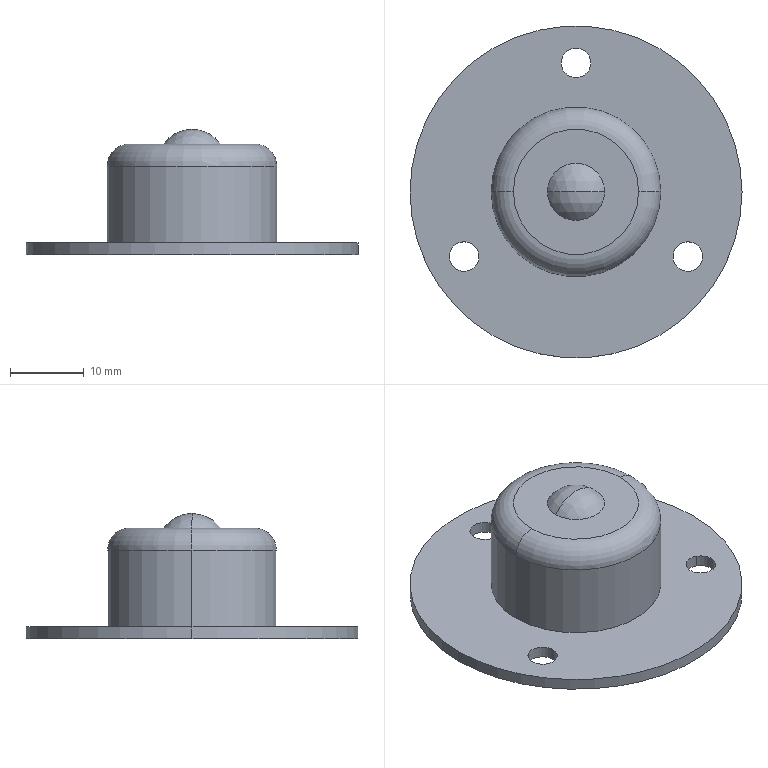Part | STEP file | Caster wheel | 1 solid | 17 faces | box 45 x 45 x 17 mm | volume 7972 mm3 | cylinder 10 | plane 3 | torus 2 | sphere 2 | commonest cylinder face diameters 4 x6 23 x2 45 x2
STEP:
#1=CARTESIAN_POINT('',(0.,0.,0.));
#2=DIRECTION('',(0.,0.,1.));
#3=DIRECTION('',(1.,0.,0.));
#4=AXIS2_PLACEMENT_3D('',#1,#2,#3);
#5=CARTESIAN_POINT('',(-16.155,-7.018,0.));
#6=VERTEX_POINT('',#5);
#7=CARTESIAN_POINT('',(-16.155,-7.018,1.6));
#8=VERTEX_POINT('',#7);
#9=CARTESIAN_POINT('',(-16.155,-7.018,1.6));
#10=DIRECTION('',(0.,0.,1.));
#11=VECTOR('',#10,1.);
#12=LINE('',#9,#11);
#13=CARTESIAN_POINT('',(-15.155,-8.75,1.6));
#14=DIRECTION('',(0.,0.,1.));
#15=DIRECTION('',(-0.5,0.866,0.));
#16=AXIS2_PLACEMENT_3D('',#13,#14,#15);
#17=CYLINDRICAL_SURFACE('',#16,2.);
#18=CARTESIAN_POINT('',(6.283,0.));
#19=DIRECTION('',(0.,1.));
#20=VECTOR('',#19,1.);
#21=LINE('',#18,#20);
#22=(GEOMETRIC_REPRESENTATION_CONTEXT(2)PARAMETRIC_REPRESENTATION_CONTEXT()REPRESENTATION_CONTEXT('',''));
#23=DEFINITIONAL_REPRESENTATION('',(#21),#22);
#24=PCURVE('',#17,#23);
#25=CARTESIAN_POINT('',(-15.155,-8.75,1.6));
#26=DIRECTION('',(0.,0.,1.));
#27=DIRECTION('',(-0.5,0.866,0.));
#28=AXIS2_PLACEMENT_3D('',#25,#26,#27);
#29=CYLINDRICAL_SURFACE('',#28,2.);
#30=CARTESIAN_POINT('',(0.,0.));
#31=DIRECTION('',(0.,1.));
#32=VECTOR('',#31,1.);
#33=LINE('',#30,#32);
#34=(GEOMETRIC_REPRESENTATION_CONTEXT(2)PARAMETRIC_REPRESENTATION_CONTEXT()REPRESENTATION_CONTEXT('',''));
#35=DEFINITIONAL_REPRESENTATION('',(#33),#34);
#36=PCURVE('',#29,#35);
#37=SURFACE_CURVE('',#12,(#24,#36),.PCURVE_S1.);
#38=EDGE_CURVE('',#6,#8,#37,.T.);
#39=ORIENTED_EDGE('',*,*,#38,.T.);
#40=CARTESIAN_POINT('',(-14.155,-10.482,1.6));
#41=VERTEX_POINT('',#40);
#42=CARTESIAN_POINT('',(-15.155,-8.75,1.6));
#43=DIRECTION('',(0.,0.,1.));
#44=DIRECTION('',(-0.5,0.866,0.));
#45=AXIS2_PLACEMENT_3D('',#42,#43,#44);
#46=CIRCLE('',#45,2.);
#47=CARTESIAN_POINT('',(0.,0.));
#48=DIRECTION('',(1.,0.));
#49=VECTOR('',#48,1.);
#50=LINE('',#47,#49);
#51=(GEOMETRIC_REPRESENTATION_CONTEXT(2)PARAMETRIC_REPRESENTATION_CONTEXT()REPRESENTATION_CONTEXT('',''));
#52=DEFINITIONAL_REPRESENTATION('',(#50),#51);
#53=PCURVE('',#17,#52);
#54=CARTESIAN_POINT('',(0.,0.,1.6));
#55=DIRECTION('',(0.,0.,1.));
#56=DIRECTION('',(1.,0.,0.));
#57=AXIS2_PLACEMENT_3D('',#54,#55,#56);
#58=PLANE('',#57);
#59=CARTESIAN_POINT('',(-15.155,-8.75));
#60=DIRECTION('',(-0.5,0.866));
#61=AXIS2_PLACEMENT_2D('',#59,#60);
#62=CIRCLE('',#61,2.);
#63=(GEOMETRIC_REPRESENTATION_CONTEXT(2)PARAMETRIC_REPRESENTATION_CONTEXT()REPRESENTATION_CONTEXT('',''));
#64=DEFINITIONAL_REPRESENTATION('',(#62),#63);
#65=PCURVE('',#58,#64);
#66=SURFACE_CURVE('',#46,(#53,#65),.PCURVE_S1.);
#67=EDGE_CURVE('',#41,#8,#66,.T.);
#68=ORIENTED_EDGE('',*,*,#67,.F.);
#69=CARTESIAN_POINT('',(-14.155,-10.482,0.));
#70=VERTEX_POINT('',#69);
#71=CARTESIAN_POINT('',(-14.155,-10.482,1.6));
#72=DIRECTION('',(0.,0.,1.));
#73=VECTOR('',#72,1.);
#74=LINE('',#71,#73);
#75=CARTESIAN_POINT('',(3.142,0.));
#76=DIRECTION('',(0.,1.));
#77=VECTOR('',#76,1.);
#78=LINE('',#75,#77);
#79=(GEOMETRIC_REPRESENTATION_CONTEXT(2)PARAMETRIC_REPRESENTATION_CONTEXT()REPRESENTATION_CONTEXT('',''));
#80=DEFINITIONAL_REPRESENTATION('',(#78),#79);
#81=PCURVE('',#17,#80);
#82=CARTESIAN_POINT('',(3.142,0.));
#83=DIRECTION('',(0.,1.));
#84=VECTOR('',#83,1.);
#85=LINE('',#82,#84);
#86=(GEOMETRIC_REPRESENTATION_CONTEXT(2)PARAMETRIC_REPRESENTATION_CONTEXT()REPRESENTATION_CONTEXT('',''));
#87=DEFINITIONAL_REPRESENTATION('',(#85),#86);
#88=PCURVE('',#29,#87);
#89=SURFACE_CURVE('',#74,(#81,#88),.PCURVE_S1.);
#90=EDGE_CURVE('',#70,#41,#89,.T.);
#91=ORIENTED_EDGE('',*,*,#90,.F.);
#92=CARTESIAN_POINT('',(-15.155,-8.75,0.));
#93=DIRECTION('',(0.,0.,1.));
#94=DIRECTION('',(-0.5,0.866,0.));
#95=AXIS2_PLACEMENT_3D('',#92,#93,#94);
#96=CIRCLE('',#95,2.);
#97=CARTESIAN_POINT('',(0.,-1.6));
#98=DIRECTION('',(1.,0.));
#99=VECTOR('',#98,1.);
#100=LINE('',#97,#99);
#101=(GEOMETRIC_REPRESENTATION_CONTEXT(2)PARAMETRIC_REPRESENTATION_CONTEXT()REPRESENTATION_CONTEXT('',''));
#102=DEFINITIONAL_REPRESENTATION('',(#100),#101);
#103=PCURVE('',#17,#102);
#104=CARTESIAN_POINT('',(0.,0.,0.));
#105=DIRECTION('',(0.,0.,1.));
#106=DIRECTION('',(1.,0.,0.));
#107=AXIS2_PLACEMENT_3D('',#104,#105,#106);
#108=PLANE('',#107);
#109=CARTESIAN_POINT('',(-15.155,-8.75));
#110=DIRECTION('',(-0.5,0.866));
#111=AXIS2_PLACEMENT_2D('',#109,#110);
#112=CIRCLE('',#111,2.);
#113=(GEOMETRIC_REPRESENTATION_CONTEXT(2)PARAMETRIC_REPRESENTATION_CONTEXT()REPRESENTATION_CONTEXT('',''));
#114=DEFINITIONAL_REPRESENTATION('',(#112),#113);
#115=PCURVE('',#108,#114);
#116=SURFACE_CURVE('',#96,(#103,#115),.PCURVE_S1.);
#117=EDGE_CURVE('',#70,#6,#116,.T.);
#118=ORIENTED_EDGE('',*,*,#117,.T.);
#119=EDGE_LOOP('',(#39,#68,#91,#118));
#120=FACE_BOUND('',#119,.F.);
#121=ADVANCED_FACE('',(#120),#17,.F.);
#122=CARTESIAN_POINT('',(14.155,-10.482,0.));
#123=VERTEX_POINT('',#122);
#124=CARTESIAN_POINT('',(14.155,-10.482,1.6));
#125=VERTEX_POINT('',#124);
#126=CARTESIAN_POINT('',(14.155,-10.482,1.6));
#127=DIRECTION('',(0.,0.,1.));
#128=VECTOR('',#127,1.);
#129=LINE('',#126,#128);
#130=CARTESIAN_POINT('',(15.155,-8.75,1.6));
#131=DIRECTION('',(0.,0.,1.));
#132=DIRECTION('',(-0.5,-0.866,0.));
#133=AXIS2_PLACEMENT_3D('',#130,#131,#132);
#134=CYLINDRICAL_SURFACE('',#133,2.);
#135=CARTESIAN_POINT('',(6.283,0.));
#136=DIRECTION('',(0.,1.));
#137=VECTOR('',#136,1.);
#138=LINE('',#135,#137);
#139=(GEOMETRIC_REPRESENTATION_CONTEXT(2)PARAMETRIC_REPRESENTATION_CONTEXT()REPRESENTATION_CONTEXT('',''));
#140=DEFINITIONAL_REPRESENTATION('',(#138),#139);
#141=PCURVE('',#134,#140);
#142=CARTESIAN_POINT('',(15.155,-8.75,1.6));
#143=DIRECTION('',(0.,0.,1.));
#144=DIRECTION('',(-0.5,-0.866,0.));
#145=AXIS2_PLACEMENT_3D('',#142,#143,#144);
#146=CYLINDRICAL_SURFACE('',#145,2.);
#147=CARTESIAN_POINT('',(0.,0.));
#148=DIRECTION('',(0.,1.));
#149=VECTOR('',#148,1.);
#150=LINE('',#147,#149);
#151=(GEOMETRIC_REPRESENTATION_CONTEXT(2)PARAMETRIC_REPRESENTATION_CONTEXT()REPRESENTATION_CONTEXT('',''));
#152=DEFINITIONAL_REPRESENTATION('',(#150),#151);
#153=PCURVE('',#146,#152);
#154=SURFACE_CURVE('',#129,(#141,#153),.PCURVE_S1.);
#155=EDGE_CURVE('',#123,#125,#154,.T.);
#156=ORIENTED_EDGE('',*,*,#155,.T.);
#157=CARTESIAN_POINT('',(16.155,-7.018,1.6));
#158=VERTEX_POINT('',#157);
#159=CARTESIAN_POINT('',(15.155,-8.75,1.6));
#160=DIRECTION('',(0.,0.,1.));
#161=DIRECTION('',(-0.5,-0.866,0.));
#162=AXIS2_PLACEMENT_3D('',#159,#160,#161);
#163=CIRCLE('',#162,2.);
#164=CARTESIAN_POINT('',(0.,0.));
#165=DIRECTION('',(1.,0.));
#166=VECTOR('',#165,1.);
#167=LINE('',#164,#166);
#168=(GEOMETRIC_REPRESENTATION_CONTEXT(2)PARAMETRIC_REPRESENTATION_CONTEXT()REPRESENTATION_CONTEXT('',''));
#169=DEFINITIONAL_REPRESENTATION('',(#167),#168);
#170=PCURVE('',#134,#169);
#171=CARTESIAN_POINT('',(15.155,-8.75));
#172=DIRECTION('',(-0.5,-0.866));
#173=AXIS2_PLACEMENT_2D('',#171,#172);
#174=CIRCLE('',#173,2.);
#175=(GEOMETRIC_REPRESENTATION_CONTEXT(2)PARAMETRIC_REPRESENTATION_CONTEXT()REPRESENTATION_CONTEXT('',''));
#176=DEFINITIONAL_REPRESENTATION('',(#174),#175);
#177=PCURVE('',#58,#176);
#178=SURFACE_CURVE('',#163,(#170,#177),.PCURVE_S1.);
#179=EDGE_CURVE('',#158,#125,#178,.T.);
#180=ORIENTED_EDGE('',*,*,#179,.F.);
#181=CARTESIAN_POINT('',(16.155,-7.018,0.));
#182=VERTEX_POINT('',#181);
#183=CARTESIAN_POINT('',(16.155,-7.018,1.6));
#184=DIRECTION('',(0.,0.,1.));
#185=VECTOR('',#184,1.);
#186=LINE('',#183,#185);
#187=CARTESIAN_POINT('',(3.142,0.));
#188=DIRECTION('',(0.,1.));
#189=VECTOR('',#188,1.);
#190=LINE('',#187,#189);
#191=(GEOMETRIC_REPRESENTATION_CONTEXT(2)PARAMETRIC_REPRESENTATION_CONTEXT()REPRESENTATION_CONTEXT('',''));
#192=DEFINITIONAL_REPRESENTATION('',(#190),#191);
#193=PCURVE('',#134,#192);
#194=CARTESIAN_POINT('',(3.142,0.));
#195=DIRECTION('',(0.,1.));
#196=VECTOR('',#195,1.);
#197=LINE('',#194,#196);
#198=(GEOMETRIC_REPRESENTATION_CONTEXT(2)PARAMETRIC_REPRESENTATION_CONTEXT()REPRESENTATION_CONTEXT('',''));
#199=DEFINITIONAL_REPRESENTATION('',(#197),#198);
#200=PCURVE('',#146,#199);
#201=SURFACE_CURVE('',#186,(#193,#200),.PCURVE_S1.);
#202=EDGE_CURVE('',#182,#158,#201,.T.);
#203=ORIENTED_EDGE('',*,*,#202,.F.);
#204=CARTESIAN_POINT('',(15.155,-8.75,0.));
#205=DIRECTION('',(0.,0.,1.));
#206=DIRECTION('',(-0.5,-0.866,0.));
#207=AXIS2_PLACEMENT_3D('',#204,#205,#206);
#208=CIRCLE('',#207,2.);
#209=CARTESIAN_POINT('',(0.,-1.6));
#210=DIRECTION('',(1.,0.));
#211=VECTOR('',#210,1.);
#212=LINE('',#209,#211);
#213=(GEOMETRIC_REPRESENTATION_CONTEXT(2)PARAMETRIC_REPRESENTATION_CONTEXT()REPRESENTATION_CONTEXT('',''));
#214=DEFINITIONAL_REPRESENTATION('',(#212),#213);
#215=PCURVE('',#134,#214);
#216=CARTESIAN_POINT('',(15.155,-8.75));
#217=DIRECTION('',(-0.5,-0.866));
#218=AXIS2_PLACEMENT_2D('',#216,#217);
#219=CIRCLE('',#218,2.);
#220=(GEOMETRIC_REPRESENTATION_CONTEXT(2)PARAMETRIC_REPRESENTATION_CONTEXT()REPRESENTATION_CONTEXT('',''));
#221=DEFINITIONAL_REPRESENTATION('',(#219),#220);
#222=PCURVE('',#108,#221);
#223=SURFACE_CURVE('',#208,(#215,#222),.PCURVE_S1.);
#224=EDGE_CURVE('',#182,#123,#223,.T.);
#225=ORIENTED_EDGE('',*,*,#224,.T.);
#226=EDGE_LOOP('',(#156,#180,#203,#225));
#227=FACE_BOUND('',#226,.F.);
#228=ADVANCED_FACE('',(#227),#134,.F.);
#229=CARTESIAN_POINT('',(2.,17.5,0.));
#230=VERTEX_POINT('',#229);
#231=CARTESIAN_POINT('',(2.,17.5,1.6));
#232=VERTEX_POINT('',#231);
#233=CARTESIAN_POINT('',(2.,17.5,1.6));
#234=DIRECTION('',(0.,0.,1.));
#235=VECTOR('',#234,1.);
#236=LINE('',#233,#235);
#237=CARTESIAN_POINT('',(0.,17.5,1.6));
#238=DIRECTION('',(0.,0.,1.));
#239=DIRECTION('',(1.,0.,0.));
#240=AXIS2_PLACEMENT_3D('',#237,#238,#239);
#241=CYLINDRICAL_SURFACE('',#240,2.);
#242=CARTESIAN_POINT('',(6.283,0.));
#243=DIRECTION('',(0.,1.));
#244=VECTOR('',#243,1.);
#245=LINE('',#242,#244);
#246=(GEOMETRIC_REPRESENTATION_CONTEXT(2)PARAMETRIC_REPRESENTATION_CONTEXT()REPRESENTATION_CONTEXT('',''));
#247=DEFINITIONAL_REPRESENTATION('',(#245),#246);
#248=PCURVE('',#241,#247);
#249=CARTESIAN_POINT('',(0.,17.5,1.6));
#250=DIRECTION('',(0.,0.,1.));
#251=DIRECTION('',(1.,0.,0.));
#252=AXIS2_PLACEMENT_3D('',#249,#250,#251);
#253=CYLINDRICAL_SURFACE('',#252,2.);
#254=CARTESIAN_POINT('',(0.,0.));
#255=DIRECTION('',(0.,1.));
#256=VECTOR('',#255,1.);
#257=LINE('',#254,#256);
#258=(GEOMETRIC_REPRESENTATION_CONTEXT(2)PARAMETRIC_REPRESENTATION_CONTEXT()REPRESENTATION_CONTEXT('',''));
#259=DEFINITIONAL_REPRESENTATION('',(#257),#258);
#260=PCURVE('',#253,#259);
#261=SURFACE_CURVE('',#236,(#248,#260),.PCURVE_S1.);
#262=EDGE_CURVE('',#230,#232,#261,.T.);
#263=ORIENTED_EDGE('',*,*,#262,.T.);
#264=CARTESIAN_POINT('',(-2.,17.5,1.6));
#265=VERTEX_POINT('',#264);
#266=CARTESIAN_POINT('',(0.,17.5,1.6));
#267=DIRECTION('',(0.,0.,1.));
#268=DIRECTION('',(1.,0.,0.));
#269=AXIS2_PLACEMENT_3D('',#266,#267,#268);
#270=CIRCLE('',#269,2.);
#271=CARTESIAN_POINT('',(0.,0.));
#272=DIRECTION('',(1.,0.));
#273=VECTOR('',#272,1.);
#274=LINE('',#271,#273);
#275=(GEOMETRIC_REPRESENTATION_CONTEXT(2)PARAMETRIC_REPRESENTATION_CONTEXT()REPRESENTATION_CONTEXT('',''));
#276=DEFINITIONAL_REPRESENTATION('',(#274),#275);
#277=PCURVE('',#241,#276);
#278=CARTESIAN_POINT('',(0.,17.5));
#279=DIRECTION('',(1.,0.));
#280=AXIS2_PLACEMENT_2D('',#278,#279);
#281=CIRCLE('',#280,2.);
#282=(GEOMETRIC_REPRESENTATION_CONTEXT(2)PARAMETRIC_REPRESENTATION_CONTEXT()REPRESENTATION_CONTEXT('',''));
#283=DEFINITIONAL_REPRESENTATION('',(#281),#282);
#284=PCURVE('',#58,#283);
#285=SURFACE_CURVE('',#270,(#277,#284),.PCURVE_S1.);
#286=EDGE_CURVE('',#265,#232,#285,.T.);
#287=ORIENTED_EDGE('',*,*,#286,.F.);
#288=CARTESIAN_POINT('',(-2.,17.5,0.));
#289=VERTEX_POINT('',#288);
#290=CARTESIAN_POINT('',(-2.,17.5,1.6));
#291=DIRECTION('',(0.,0.,1.));
#292=VECTOR('',#291,1.);
#293=LINE('',#290,#292);
#294=CARTESIAN_POINT('',(3.142,0.));
#295=DIRECTION('',(0.,1.));
#296=VECTOR('',#295,1.);
#297=LINE('',#294,#296);
#298=(GEOMETRIC_REPRESENTATION_CONTEXT(2)PARAMETRIC_REPRESENTATION_CONTEXT()REPRESENTATION_CONTEXT('',''));
#299=DEFINITIONAL_REPRESENTATION('',(#297),#298);
#300=PCURVE('',#241,#299);
#301=CARTESIAN_POINT('',(3.142,0.));
#302=DIRECTION('',(0.,1.));
#303=VECTOR('',#302,1.);
#304=LINE('',#301,#303);
#305=(GEOMETRIC_REPRESENTATION_CONTEXT(2)PARAMETRIC_REPRESENTATION_CONTEXT()REPRESENTATION_CONTEXT('',''));
#306=DEFINITIONAL_REPRESENTATION('',(#304),#305);
#307=PCURVE('',#253,#306);
#308=SURFACE_CURVE('',#293,(#300,#307),.PCURVE_S1.);
#309=EDGE_CURVE('',#289,#265,#308,.T.);
#310=ORIENTED_EDGE('',*,*,#309,.F.);
#311=CARTESIAN_POINT('',(0.,17.5,0.));
#312=DIRECTION('',(0.,0.,1.));
#313=DIRECTION('',(1.,0.,0.));
#314=AXIS2_PLACEMENT_3D('',#311,#312,#313);
#315=CIRCLE('',#314,2.);
#316=CARTESIAN_POINT('',(0.,-1.6));
#317=DIRECTION('',(1.,0.));
#318=VECTOR('',#317,1.);
#319=LINE('',#316,#318);
#320=(GEOMETRIC_REPRESENTATION_CONTEXT(2)PARAMETRIC_REPRESENTATION_CONTEXT()REPRESENTATION_CONTEXT('',''));
#321=DEFINITIONAL_REPRESENTATION('',(#319),#320);
#322=PCURVE('',#241,#321);
#323=CARTESIAN_POINT('',(0.,17.5));
#324=DIRECTION('',(1.,0.));
#325=AXIS2_PLACEMENT_2D('',#323,#324);
#326=CIRCLE('',#325,2.);
#327=(GEOMETRIC_REPRESENTATION_CONTEXT(2)PARAMETRIC_REPRESENTATION_CONTEXT()REPRESENTATION_CONTEXT('',''));
#328=DEFINITIONAL_REPRESENTATION('',(#326),#327);
#329=PCURVE('',#108,#328);
#330=SURFACE_CURVE('',#315,(#322,#329),.PCURVE_S1.);
#331=EDGE_CURVE('',#289,#230,#330,.T.);
#332=ORIENTED_EDGE('',*,*,#331,.T.);
#333=EDGE_LOOP('',(#263,#287,#310,#332));
#334=FACE_BOUND('',#333,.F.);
#335=ADVANCED_FACE('',(#334),#241,.F.);
#336=CARTESIAN_POINT('',(8.5,0.,15.));
#337=VERTEX_POINT('',#336);
#338=CARTESIAN_POINT('',(-8.5,0.,15.));
#339=VERTEX_POINT('',#338);
#340=CARTESIAN_POINT('',(0.,0.,15.));
#341=DIRECTION('',(0.,0.,1.));
#342=DIRECTION('',(-1.,0.,0.));
#343=AXIS2_PLACEMENT_3D('',#340,#341,#342);
#344=CIRCLE('',#343,8.5);
#345=CARTESIAN_POINT('',(0.,0.,12.));
#346=DIRECTION('',(0.,0.,-1.));
#347=DIRECTION('',(-1.,0.,0.));
#348=AXIS2_PLACEMENT_3D('',#345,#346,#347);
#349=TOROIDAL_SURFACE('',#348,8.5,3.);
#350=CARTESIAN_POINT('',(6.283,4.712));
#351=DIRECTION('',(-1.,0.));
#352=VECTOR('',#351,1.);
#353=LINE('',#350,#352);
#354=(GEOMETRIC_REPRESENTATION_CONTEXT(2)PARAMETRIC_REPRESENTATION_CONTEXT()REPRESENTATION_CONTEXT('',''));
#355=DEFINITIONAL_REPRESENTATION('',(#353),#354);
#356=PCURVE('',#349,#355);
#357=CARTESIAN_POINT('',(-11.5,0.,15.));
#358=DIRECTION('',(0.,0.,-1.));
#359=DIRECTION('',(-1.,0.,0.));
#360=AXIS2_PLACEMENT_3D('',#357,#358,#359);
#361=PLANE('',#360);
#362=CARTESIAN_POINT('',(-3.,0.));
#363=CARTESIAN_POINT('',(-3.,-14.722));
#364=CARTESIAN_POINT('',(-15.75,-7.361));
#365=CARTESIAN_POINT('',(-28.5,0.));
#366=CARTESIAN_POINT('',(-15.75,7.361));
#367=CARTESIAN_POINT('',(-3.,14.722));
#368=CARTESIAN_POINT('',(-3.,0.));
#369=(BOUNDED_CURVE()B_SPLINE_CURVE(2,(#362,#363,#364,#365,#366,#367,#368),.UNSPECIFIED.,.T.,.F.)B_SPLINE_CURVE_WITH_KNOTS((1,2,2,2,2,1),(-2.094,0.,2.094,4.189,6.283,8.378),.UNSPECIFIED.)CURVE()GEOMETRIC_REPRESENTATION_ITEM()RATIONAL_B_SPLINE_CURVE((1.,0.5,1.,0.5,1.,0.5,1.))REPRESENTATION_ITEM(''));
#370=(GEOMETRIC_REPRESENTATION_CONTEXT(2)PARAMETRIC_REPRESENTATION_CONTEXT()REPRESENTATION_CONTEXT('',''));
#371=DEFINITIONAL_REPRESENTATION('',(#369),#370);
#372=PCURVE('',#361,#371);
#373=SURFACE_CURVE('',#344,(#356,#372),.PCURVE_S1.);
#374=EDGE_CURVE('',#337,#339,#373,.T.);
#375=ORIENTED_EDGE('',*,*,#374,.F.);
#376=CARTESIAN_POINT('',(11.5,0.,12.));
#377=VERTEX_POINT('',#376);
#378=CARTESIAN_POINT('',(8.5,0.,12.));
#379=DIRECTION('',(0.,1.,0.));
#380=DIRECTION('',(-1.,0.,0.));
#381=AXIS2_PLACEMENT_3D('',#378,#379,#380);
#382=CIRCLE('',#381,3.);
#383=CARTESIAN_POINT('',(3.142,3.142));
#384=DIRECTION('',(0.,1.));
#385=VECTOR('',#384,1.);
#386=LINE('',#383,#385);
#387=(GEOMETRIC_REPRESENTATION_CONTEXT(2)PARAMETRIC_REPRESENTATION_CONTEXT()REPRESENTATION_CONTEXT('',''));
#388=DEFINITIONAL_REPRESENTATION('',(#386),#387);
#389=PCURVE('',#349,#388);
#390=CARTESIAN_POINT('',(0.,0.,12.));
#391=DIRECTION('',(0.,0.,-1.));
#392=DIRECTION('',(-1.,0.,0.));
#393=AXIS2_PLACEMENT_3D('',#390,#391,#392);
#394=TOROIDAL_SURFACE('',#393,8.5,3.);
#395=CARTESIAN_POINT('',(3.142,3.142));
#396=DIRECTION('',(0.,1.));
#397=VECTOR('',#396,1.);
#398=LINE('',#395,#397);
#399=(GEOMETRIC_REPRESENTATION_CONTEXT(2)PARAMETRIC_REPRESENTATION_CONTEXT()REPRESENTATION_CONTEXT('',''));
#400=DEFINITIONAL_REPRESENTATION('',(#398),#399);
#401=PCURVE('',#394,#400);
#402=SURFACE_CURVE('',#382,(#389,#401),.PCURVE_S1.);
#403=EDGE_CURVE('',#337,#377,#402,.T.);
#404=ORIENTED_EDGE('',*,*,#403,.T.);
#405=CARTESIAN_POINT('',(-11.5,0.,12.));
#406=VERTEX_POINT('',#405);
#407=CARTESIAN_POINT('',(0.,0.,12.));
#408=DIRECTION('',(0.,0.,-1.));
#409=DIRECTION('',(-1.,0.,0.));
#410=AXIS2_PLACEMENT_3D('',#407,#408,#409);
#411=CIRCLE('',#410,11.5);
#412=CARTESIAN_POINT('',(0.,6.283));
#413=DIRECTION('',(1.,0.));
#414=VECTOR('',#413,1.);
#415=LINE('',#412,#414);
#416=(GEOMETRIC_REPRESENTATION_CONTEXT(2)PARAMETRIC_REPRESENTATION_CONTEXT()REPRESENTATION_CONTEXT('',''));
#417=DEFINITIONAL_REPRESENTATION('',(#415),#416);
#418=PCURVE('',#349,#417);
#419=CARTESIAN_POINT('',(0.,0.,1000.));
#420=DIRECTION('',(0.,0.,1.));
#421=DIRECTION('',(1.,0.,0.));
#422=AXIS2_PLACEMENT_3D('',#419,#420,#421);
#423=CYLINDRICAL_SURFACE('',#422,11.5);
#424=CARTESIAN_POINT('',(3.142,-988.));
#425=DIRECTION('',(-1.,0.));
#426=VECTOR('',#425,1.);
#427=LINE('',#424,#426);
#428=(GEOMETRIC_REPRESENTATION_CONTEXT(2)PARAMETRIC_REPRESENTATION_CONTEXT()REPRESENTATION_CONTEXT('',''));
#429=DEFINITIONAL_REPRESENTATION('',(#427),#428);
#430=PCURVE('',#423,#429);
#431=SURFACE_CURVE('',#411,(#418,#430),.PCURVE_S1.);
#432=EDGE_CURVE('',#406,#377,#431,.T.);
#433=ORIENTED_EDGE('',*,*,#432,.F.);
#434=CARTESIAN_POINT('',(-8.5,0.,12.));
#435=DIRECTION('',(0.,-1.,0.));
#436=DIRECTION('',(0.,0.,-1.));
#437=AXIS2_PLACEMENT_3D('',#434,#435,#436);
#438=CIRCLE('',#437,3.);
#439=CARTESIAN_POINT('',(0.,1.571));
#440=DIRECTION('',(0.,1.));
#441=VECTOR('',#440,1.);
#442=LINE('',#439,#441);
#443=(GEOMETRIC_REPRESENTATION_CONTEXT(2)PARAMETRIC_REPRESENTATION_CONTEXT()REPRESENTATION_CONTEXT('',''));
#444=DEFINITIONAL_REPRESENTATION('',(#442),#443);
#445=PCURVE('',#349,#444);
#446=CARTESIAN_POINT('',(6.283,1.571));
#447=DIRECTION('',(0.,1.));
#448=VECTOR('',#447,1.);
#449=LINE('',#446,#448);
#450=(GEOMETRIC_REPRESENTATION_CONTEXT(2)PARAMETRIC_REPRESENTATION_CONTEXT()REPRESENTATION_CONTEXT('',''));
#451=DEFINITIONAL_REPRESENTATION('',(#449),#450);
#452=PCURVE('',#394,#451);
#453=SURFACE_CURVE('',#438,(#445,#452),.PCURVE_S1.);
#454=EDGE_CURVE('',#339,#406,#453,.T.);
#455=ORIENTED_EDGE('',*,*,#454,.F.);
#456=EDGE_LOOP('',(#375,#404,#433,#455));
#457=FACE_BOUND('',#456,.T.);
#458=ADVANCED_FACE('',(#457),#349,.T.);
#459=CARTESIAN_POINT('',(-3.879,0.,15.));
#460=VERTEX_POINT('',#459);
#461=CARTESIAN_POINT('',(3.879,0.,15.));
#462=VERTEX_POINT('',#461);
#463=CARTESIAN_POINT('',(0.,0.,15.));
#464=DIRECTION('',(0.,0.,1.));
#465=DIRECTION('',(1.,0.,0.));
#466=AXIS2_PLACEMENT_3D('',#463,#464,#465);
#467=CIRCLE('',#466,3.879);
#468=CARTESIAN_POINT('',(0.,0.,12.238));
#469=DIRECTION('',(0.,-1.,0.));
#470=DIRECTION('',(-1.,0.,0.));
#471=AXIS2_PLACEMENT_3D('',#468,#469,#470);
#472=SPHERICAL_SURFACE('',#471,4.763);
#473=CARTESIAN_POINT('',(5.664,0.));
#474=CARTESIAN_POINT('',(5.664,0.03877));
#475=CARTESIAN_POINT('',(5.661,0.1163));
#476=CARTESIAN_POINT('',(5.647,0.2318));
#477=CARTESIAN_POINT('',(5.621,0.3457));
#478=CARTESIAN_POINT('',(5.583,0.4567));
#479=CARTESIAN_POINT('',(5.531,0.5637));
#480=CARTESIAN_POINT('',(5.46,0.6646));
#481=CARTESIAN_POINT('',(5.366,0.757));
#482=CARTESIAN_POINT('',(5.246,0.8373));
#483=CARTESIAN_POINT('',(5.094,0.9009));
#484=CARTESIAN_POINT('',(4.913,0.9423));
#485=CARTESIAN_POINT('',(4.712,0.9568));
#486=CARTESIAN_POINT('',(4.512,0.9423));
#487=CARTESIAN_POINT('',(4.331,0.9009));
#488=CARTESIAN_POINT('',(4.179,0.8373));
#489=CARTESIAN_POINT('',(4.058,0.757));
#490=CARTESIAN_POINT('',(3.965,0.6646));
#491=CARTESIAN_POINT('',(3.894,0.5637));
#492=CARTESIAN_POINT('',(3.842,0.4567));
#493=CARTESIAN_POINT('',(3.804,0.3457));
#494=CARTESIAN_POINT('',(3.778,0.2318));
#495=CARTESIAN_POINT('',(3.764,0.1163));
#496=CARTESIAN_POINT('',(3.76,0.03877));
#497=CARTESIAN_POINT('',(3.76,0.));
#498=B_SPLINE_CURVE_WITH_KNOTS('',3,(#473,#474,#475,#476,#477,#478,#479,#480,#481,#482,#483,#484,#485,#486,#487,#488,#489,#490,#491,#492,#493,#494,#495,#496,#497),.UNSPECIFIED.,.F.,.F.,(4,1,1,1,1,1,1,1,1,1,1,1,1,1,1,1,1,1,1,1,1,1,4),(3.142,3.284,3.427,3.57,3.713,3.856,3.998,4.141,4.284,4.427,4.57,4.712,4.855,4.998,5.141,5.284,5.426,5.569,5.712,5.855,5.998,6.14,6.283),.QUASI_UNIFORM_KNOTS.);
#499=(GEOMETRIC_REPRESENTATION_CONTEXT(2)PARAMETRIC_REPRESENTATION_CONTEXT()REPRESENTATION_CONTEXT('',''));
#500=DEFINITIONAL_REPRESENTATION('',(#498),#499);
#501=PCURVE('',#472,#500);
#502=CARTESIAN_POINT('',(-15.379,0.));
#503=CARTESIAN_POINT('',(-15.379,6.719));
#504=CARTESIAN_POINT('',(-9.56,3.36));
#505=CARTESIAN_POINT('',(-3.741,0.));
#506=CARTESIAN_POINT('',(-9.56,-3.36));
#507=CARTESIAN_POINT('',(-15.379,-6.719));
#508=CARTESIAN_POINT('',(-15.379,0.));
#509=(BOUNDED_CURVE()B_SPLINE_CURVE(2,(#502,#503,#504,#505,#506,#507,#508),.UNSPECIFIED.,.T.,.F.)B_SPLINE_CURVE_WITH_KNOTS((1,2,2,2,2,1),(-2.094,0.,2.094,4.189,6.283,8.378),.UNSPECIFIED.)CURVE()GEOMETRIC_REPRESENTATION_ITEM()RATIONAL_B_SPLINE_CURVE((1.,0.5,1.,0.5,1.,0.5,1.))REPRESENTATION_ITEM(''));
#510=(GEOMETRIC_REPRESENTATION_CONTEXT(2)PARAMETRIC_REPRESENTATION_CONTEXT()REPRESENTATION_CONTEXT('',''));
#511=DEFINITIONAL_REPRESENTATION('',(#509),#510);
#512=PCURVE('',#361,#511);
#513=SURFACE_CURVE('',#467,(#501,#512),.PCURVE_S1.);
#514=EDGE_CURVE('',#460,#462,#513,.T.);
#515=ORIENTED_EDGE('',*,*,#514,.T.);
#516=CARTESIAN_POINT('',(0.,0.,17.));
#517=VERTEX_POINT('',#516);
#518=CARTESIAN_POINT('',(0.,0.,12.238));
#519=DIRECTION('',(0.,-1.,0.));
#520=DIRECTION('',(1.,0.,0.));
#521=AXIS2_PLACEMENT_3D('',#518,#519,#520);
#522=CIRCLE('',#521,4.763);
#523=CARTESIAN_POINT('',(3.142,0.));
#524=DIRECTION('',(1.,0.));
#525=VECTOR('',#524,1.);
#526=LINE('',#523,#525);
#527=(GEOMETRIC_REPRESENTATION_CONTEXT(2)PARAMETRIC_REPRESENTATION_CONTEXT()REPRESENTATION_CONTEXT('',''));
#528=DEFINITIONAL_REPRESENTATION('',(#526),#527);
#529=PCURVE('',#472,#528);
#530=CARTESIAN_POINT('',(0.,0.,12.238));
#531=DIRECTION('',(0.,-1.,0.));
#532=DIRECTION('',(-1.,0.,0.));
#533=AXIS2_PLACEMENT_3D('',#530,#531,#532);
#534=SPHERICAL_SURFACE('',#533,4.763);
#535=CARTESIAN_POINT('',(3.142,0.));
#536=DIRECTION('',(1.,0.));
#537=VECTOR('',#536,1.);
#538=LINE('',#535,#537);
#539=(GEOMETRIC_REPRESENTATION_CONTEXT(2)PARAMETRIC_REPRESENTATION_CONTEXT()REPRESENTATION_CONTEXT('',''));
#540=DEFINITIONAL_REPRESENTATION('',(#538),#539);
#541=PCURVE('',#534,#540);
#542=SURFACE_CURVE('',#522,(#529,#541),.PCURVE_S1.);
#543=EDGE_CURVE('',#462,#517,#542,.T.);
#544=ORIENTED_EDGE('',*,*,#543,.T.);
#545=CARTESIAN_POINT('',(0.,0.,12.238));
#546=DIRECTION('',(0.,1.,0.));
#547=DIRECTION('',(0.,0.,1.));
#548=AXIS2_PLACEMENT_3D('',#545,#546,#547);
#549=CIRCLE('',#548,4.763);
#550=CARTESIAN_POINT('',(10.996,0.));
#551=DIRECTION('',(-1.,0.));
#552=VECTOR('',#551,1.);
#553=LINE('',#550,#552);
#554=(GEOMETRIC_REPRESENTATION_CONTEXT(2)PARAMETRIC_REPRESENTATION_CONTEXT()REPRESENTATION_CONTEXT('',''));
#555=DEFINITIONAL_REPRESENTATION('',(#553),#554);
#556=PCURVE('',#472,#555);
#557=CARTESIAN_POINT('',(10.996,0.));
#558=DIRECTION('',(-1.,0.));
#559=VECTOR('',#558,1.);
#560=LINE('',#557,#559);
#561=(GEOMETRIC_REPRESENTATION_CONTEXT(2)PARAMETRIC_REPRESENTATION_CONTEXT()REPRESENTATION_CONTEXT('',''));
#562=DEFINITIONAL_REPRESENTATION('',(#560),#561);
#563=PCURVE('',#534,#562);
#564=SURFACE_CURVE('',#549,(#556,#563),.PCURVE_S1.);
#565=EDGE_CURVE('',#460,#517,#564,.T.);
#566=ORIENTED_EDGE('',*,*,#565,.F.);
#567=EDGE_LOOP('',(#515,#544,#566));
#568=FACE_BOUND('',#567,.T.);
#569=ADVANCED_FACE('',(#568),#472,.T.);
#570=CARTESIAN_POINT('',(11.5,0.,1.6));
#571=VERTEX_POINT('',#570);
#572=CARTESIAN_POINT('',(-11.5,0.,1.6));
#573=VERTEX_POINT('',#572);
#574=CARTESIAN_POINT('',(0.,0.,1.6));
#575=DIRECTION('',(0.,0.,1.));
#576=DIRECTION('',(1.,0.,0.));
#577=AXIS2_PLACEMENT_3D('',#574,#575,#576);
#578=CIRCLE('',#577,11.5);
#579=CARTESIAN_POINT('',(0.,-998.4));
#580=DIRECTION('',(1.,0.));
#581=VECTOR('',#580,1.);
#582=LINE('',#579,#581);
#583=(GEOMETRIC_REPRESENTATION_CONTEXT(2)PARAMETRIC_REPRESENTATION_CONTEXT()REPRESENTATION_CONTEXT('',''));
#584=DEFINITIONAL_REPRESENTATION('',(#582),#583);
#585=PCURVE('',#423,#584);
#586=CARTESIAN_POINT('',(0.,0.));
#587=DIRECTION('',(1.,0.));
#588=AXIS2_PLACEMENT_2D('',#586,#587);
#589=CIRCLE('',#588,11.5);
#590=(GEOMETRIC_REPRESENTATION_CONTEXT(2)PARAMETRIC_REPRESENTATION_CONTEXT()REPRESENTATION_CONTEXT('',''));
#591=DEFINITIONAL_REPRESENTATION('',(#589),#590);
#592=PCURVE('',#58,#591);
#593=SURFACE_CURVE('',#578,(#585,#592),.PCURVE_S1.);
#594=EDGE_CURVE('',#571,#573,#593,.T.);
#595=ORIENTED_EDGE('',*,*,#594,.T.);
#596=CARTESIAN_POINT('',(-11.5,0.,1000.));
#597=DIRECTION('',(0.,0.,1.));
#598=VECTOR('',#597,1.);
#599=LINE('',#596,#598);
#600=CARTESIAN_POINT('',(3.142,0.));
#601=DIRECTION('',(0.,1.));
#602=VECTOR('',#601,1.);
#603=LINE('',#600,#602);
#604=(GEOMETRIC_REPRESENTATION_CONTEXT(2)PARAMETRIC_REPRESENTATION_CONTEXT()REPRESENTATION_CONTEXT('',''));
#605=DEFINITIONAL_REPRESENTATION('',(#603),#604);
#606=PCURVE('',#423,#605);
#607=CARTESIAN_POINT('',(0.,0.,1000.));
#608=DIRECTION('',(0.,0.,1.));
#609=DIRECTION('',(1.,0.,0.));
#610=AXIS2_PLACEMENT_3D('',#607,#608,#609);
#611=CYLINDRICAL_SURFACE('',#610,11.5);
#612=CARTESIAN_POINT('',(3.142,0.));
#613=DIRECTION('',(0.,1.));
#614=VECTOR('',#613,1.);
#615=LINE('',#612,#614);
#616=(GEOMETRIC_REPRESENTATION_CONTEXT(2)PARAMETRIC_REPRESENTATION_CONTEXT()REPRESENTATION_CONTEXT('',''));
#617=DEFINITIONAL_REPRESENTATION('',(#615),#616);
#618=PCURVE('',#611,#617);
#619=SURFACE_CURVE('',#599,(#606,#618),.PCURVE_S1.);
#620=EDGE_CURVE('',#573,#406,#619,.T.);
#621=ORIENTED_EDGE('',*,*,#620,.T.);
#622=ORIENTED_EDGE('',*,*,#432,.T.);
#623=CARTESIAN_POINT('',(11.5,0.,1000.));
#624=DIRECTION('',(0.,0.,1.));
#625=VECTOR('',#624,1.);
#626=LINE('',#623,#625);
#627=CARTESIAN_POINT('',(0.,0.));
#628=DIRECTION('',(0.,1.));
#629=VECTOR('',#628,1.);
#630=LINE('',#627,#629);
#631=(GEOMETRIC_REPRESENTATION_CONTEXT(2)PARAMETRIC_REPRESENTATION_CONTEXT()REPRESENTATION_CONTEXT('',''));
#632=DEFINITIONAL_REPRESENTATION('',(#630),#631);
#633=PCURVE('',#423,#632);
#634=CARTESIAN_POINT('',(6.283,0.));
#635=DIRECTION('',(0.,1.));
#636=VECTOR('',#635,1.);
#637=LINE('',#634,#636);
#638=(GEOMETRIC_REPRESENTATION_CONTEXT(2)PARAMETRIC_REPRESENTATION_CONTEXT()REPRESENTATION_CONTEXT('',''));
#639=DEFINITIONAL_REPRESENTATION('',(#637),#638);
#640=PCURVE('',#611,#639);
#641=SURFACE_CURVE('',#626,(#633,#640),.PCURVE_S1.);
#642=EDGE_CURVE('',#571,#377,#641,.T.);
#643=ORIENTED_EDGE('',*,*,#642,.F.);
#644=EDGE_LOOP('',(#595,#621,#622,#643));
#645=FACE_BOUND('',#644,.T.);
#646=ADVANCED_FACE('',(#645),#423,.T.);
#647=CARTESIAN_POINT('',(22.5,0.,1.6));
#648=VERTEX_POINT('',#647);
#649=CARTESIAN_POINT('',(-22.5,0.,1.6));
#650=VERTEX_POINT('',#649);
#651=CARTESIAN_POINT('',(0.,0.,1.6));
#652=DIRECTION('',(0.,0.,1.));
#653=DIRECTION('',(1.,0.,0.));
#654=AXIS2_PLACEMENT_3D('',#651,#652,#653);
#655=CIRCLE('',#654,22.5);
#656=CARTESIAN_POINT('',(0.,0.,1.6));
#657=DIRECTION('',(0.,0.,-1.));
#658=DIRECTION('',(-1.,0.,0.));
#659=AXIS2_PLACEMENT_3D('',#656,#657,#658);
#660=CYLINDRICAL_SURFACE('',#659,22.5);
#661=CARTESIAN_POINT('',(3.142,0.));
#662=DIRECTION('',(-1.,0.));
#663=VECTOR('',#662,1.);
#664=LINE('',#661,#663);
#665=(GEOMETRIC_REPRESENTATION_CONTEXT(2)PARAMETRIC_REPRESENTATION_CONTEXT()REPRESENTATION_CONTEXT('',''));
#666=DEFINITIONAL_REPRESENTATION('',(#664),#665);
#667=PCURVE('',#660,#666);
#668=CARTESIAN_POINT('',(0.,0.));
#669=DIRECTION('',(1.,0.));
#670=AXIS2_PLACEMENT_2D('',#668,#669);
#671=CIRCLE('',#670,22.5);
#672=(GEOMETRIC_REPRESENTATION_CONTEXT(2)PARAMETRIC_REPRESENTATION_CONTEXT()REPRESENTATION_CONTEXT('',''));
#673=DEFINITIONAL_REPRESENTATION('',(#671),#672);
#674=PCURVE('',#58,#673);
#675=SURFACE_CURVE('',#655,(#667,#674),.PCURVE_S1.);
#676=EDGE_CURVE('',#648,#650,#675,.T.);
#677=ORIENTED_EDGE('',*,*,#676,.F.);
#678=CARTESIAN_POINT('',(22.5,0.,0.));
#679=VERTEX_POINT('',#678);
#680=CARTESIAN_POINT('',(22.5,0.,1.6));
#681=DIRECTION('',(0.,0.,-1.));
#682=VECTOR('',#681,1.);
#683=LINE('',#680,#682);
#684=CARTESIAN_POINT('',(3.142,0.));
#685=DIRECTION('',(0.,1.));
#686=VECTOR('',#685,1.);
#687=LINE('',#684,#686);
#688=(GEOMETRIC_REPRESENTATION_CONTEXT(2)PARAMETRIC_REPRESENTATION_CONTEXT()REPRESENTATION_CONTEXT('',''));
#689=DEFINITIONAL_REPRESENTATION('',(#687),#688);
#690=PCURVE('',#660,#689);
#691=CARTESIAN_POINT('',(0.,0.,1.6));
#692=DIRECTION('',(0.,0.,-1.));
#693=DIRECTION('',(-1.,0.,0.));
#694=AXIS2_PLACEMENT_3D('',#691,#692,#693);
#695=CYLINDRICAL_SURFACE('',#694,22.5);
#696=CARTESIAN_POINT('',(3.142,0.));
#697=DIRECTION('',(0.,1.));
#698=VECTOR('',#697,1.);
#699=LINE('',#696,#698);
#700=(GEOMETRIC_REPRESENTATION_CONTEXT(2)PARAMETRIC_REPRESENTATION_CONTEXT()REPRESENTATION_CONTEXT('',''));
#701=DEFINITIONAL_REPRESENTATION('',(#699),#700);
#702=PCURVE('',#695,#701);
#703=SURFACE_CURVE('',#683,(#690,#702),.PCURVE_S1.);
#704=EDGE_CURVE('',#648,#679,#703,.T.);
#705=ORIENTED_EDGE('',*,*,#704,.T.);
#706=CARTESIAN_POINT('',(-22.5,0.,0.));
#707=VERTEX_POINT('',#706);
#708=CARTESIAN_POINT('',(0.,0.,0.));
#709=DIRECTION('',(0.,0.,1.));
#710=DIRECTION('',(1.,0.,0.));
#711=AXIS2_PLACEMENT_3D('',#708,#709,#710);
#712=CIRCLE('',#711,22.5);
#713=CARTESIAN_POINT('',(3.142,1.6));
#714=DIRECTION('',(-1.,0.));
#715=VECTOR('',#714,1.);
#716=LINE('',#713,#715);
#717=(GEOMETRIC_REPRESENTATION_CONTEXT(2)PARAMETRIC_REPRESENTATION_CONTEXT()REPRESENTATION_CONTEXT('',''));
#718=DEFINITIONAL_REPRESENTATION('',(#716),#717);
#719=PCURVE('',#660,#718);
#720=CARTESIAN_POINT('',(0.,0.));
#721=DIRECTION('',(1.,0.));
#722=AXIS2_PLACEMENT_2D('',#720,#721);
#723=CIRCLE('',#722,22.5);
#724=(GEOMETRIC_REPRESENTATION_CONTEXT(2)PARAMETRIC_REPRESENTATION_CONTEXT()REPRESENTATION_CONTEXT('',''));
#725=DEFINITIONAL_REPRESENTATION('',(#723),#724);
#726=PCURVE('',#108,#725);
#727=SURFACE_CURVE('',#712,(#719,#726),.PCURVE_S1.);
#728=EDGE_CURVE('',#679,#707,#727,.T.);
#729=ORIENTED_EDGE('',*,*,#728,.T.);
#730=CARTESIAN_POINT('',(-22.5,0.,1.6));
#731=DIRECTION('',(0.,0.,-1.));
#732=VECTOR('',#731,1.);
#733=LINE('',#730,#732);
#734=CARTESIAN_POINT('',(0.,0.));
#735=DIRECTION('',(0.,1.));
#736=VECTOR('',#735,1.);
#737=LINE('',#734,#736);
#738=(GEOMETRIC_REPRESENTATION_CONTEXT(2)PARAMETRIC_REPRESENTATION_CONTEXT()REPRESENTATION_CONTEXT('',''));
#739=DEFINITIONAL_REPRESENTATION('',(#737),#738);
#740=PCURVE('',#660,#739);
#741=CARTESIAN_POINT('',(6.283,0.));
#742=DIRECTION('',(0.,1.));
#743=VECTOR('',#742,1.);
#744=LINE('',#741,#743);
#745=(GEOMETRIC_REPRESENTATION_CONTEXT(2)PARAMETRIC_REPRESENTATION_CONTEXT()REPRESENTATION_CONTEXT('',''));
#746=DEFINITIONAL_REPRESENTATION('',(#744),#745);
#747=PCURVE('',#695,#746);
#748=SURFACE_CURVE('',#733,(#740,#747),.PCURVE_S1.);
#749=EDGE_CURVE('',#650,#707,#748,.T.);
#750=ORIENTED_EDGE('',*,*,#749,.F.);
#751=EDGE_LOOP('',(#677,#705,#729,#750));
#752=FACE_BOUND('',#751,.T.);
#753=ADVANCED_FACE('',(#752),#660,.T.);
#754=CARTESIAN_POINT('',(-15.155,-8.75,1.6));
#755=DIRECTION('',(0.,0.,1.));
#756=DIRECTION('',(-0.5,0.866,0.));
#757=AXIS2_PLACEMENT_3D('',#754,#755,#756);
#758=CIRCLE('',#757,2.);
#759=CARTESIAN_POINT('',(-15.155,-8.75));
#760=DIRECTION('',(-0.5,0.866));
#761=AXIS2_PLACEMENT_2D('',#759,#760);
#762=CIRCLE('',#761,2.);
#763=(GEOMETRIC_REPRESENTATION_CONTEXT(2)PARAMETRIC_REPRESENTATION_CONTEXT()REPRESENTATION_CONTEXT('',''));
#764=DEFINITIONAL_REPRESENTATION('',(#762),#763);
#765=PCURVE('',#58,#764);
#766=CARTESIAN_POINT('',(0.,0.));
#767=DIRECTION('',(1.,0.));
#768=VECTOR('',#767,1.);
#769=LINE('',#766,#768);
#770=(GEOMETRIC_REPRESENTATION_CONTEXT(2)PARAMETRIC_REPRESENTATION_CONTEXT()REPRESENTATION_CONTEXT('',''));
#771=DEFINITIONAL_REPRESENTATION('',(#769),#770);
#772=PCURVE('',#29,#771);
#773=SURFACE_CURVE('',#758,(#765,#772),.PCURVE_S1.);
#774=EDGE_CURVE('',#8,#41,#773,.T.);
#775=ORIENTED_EDGE('',*,*,#774,.F.);
#776=ORIENTED_EDGE('',*,*,#67,.F.);
#777=EDGE_LOOP('',(#775,#776));
#778=FACE_BOUND('',#777,.T.);
#779=CARTESIAN_POINT('',(15.155,-8.75,1.6));
#780=DIRECTION('',(0.,0.,1.));
#781=DIRECTION('',(-0.5,-0.866,0.));
#782=AXIS2_PLACEMENT_3D('',#779,#780,#781);
#783=CIRCLE('',#782,2.);
#784=CARTESIAN_POINT('',(15.155,-8.75));
#785=DIRECTION('',(-0.5,-0.866));
#786=AXIS2_PLACEMENT_2D('',#784,#785);
#787=CIRCLE('',#786,2.);
#788=(GEOMETRIC_REPRESENTATION_CONTEXT(2)PARAMETRIC_REPRESENTATION_CONTEXT()REPRESENTATION_CONTEXT('',''));
#789=DEFINITIONAL_REPRESENTATION('',(#787),#788);
#790=PCURVE('',#58,#789);
#791=CARTESIAN_POINT('',(0.,0.));
#792=DIRECTION('',(1.,0.));
#793=VECTOR('',#792,1.);
#794=LINE('',#791,#793);
#795=(GEOMETRIC_REPRESENTATION_CONTEXT(2)PARAMETRIC_REPRESENTATION_CONTEXT()REPRESENTATION_CONTEXT('',''));
#796=DEFINITIONAL_REPRESENTATION('',(#794),#795);
#797=PCURVE('',#146,#796);
#798=SURFACE_CURVE('',#783,(#790,#797),.PCURVE_S1.);
#799=EDGE_CURVE('',#125,#158,#798,.T.);
#800=ORIENTED_EDGE('',*,*,#799,.F.);
#801=ORIENTED_EDGE('',*,*,#179,.F.);
#802=EDGE_LOOP('',(#800,#801));
#803=FACE_BOUND('',#802,.T.);
#804=CARTESIAN_POINT('',(0.,17.5,1.6));
#805=DIRECTION('',(0.,0.,1.));
#806=DIRECTION('',(1.,0.,0.));
#807=AXIS2_PLACEMENT_3D('',#804,#805,#806);
#808=CIRCLE('',#807,2.);
#809=CARTESIAN_POINT('',(0.,17.5));
#810=DIRECTION('',(1.,0.));
#811=AXIS2_PLACEMENT_2D('',#809,#810);
#812=CIRCLE('',#811,2.);
#813=(GEOMETRIC_REPRESENTATION_CONTEXT(2)PARAMETRIC_REPRESENTATION_CONTEXT()REPRESENTATION_CONTEXT('',''));
#814=DEFINITIONAL_REPRESENTATION('',(#812),#813);
#815=PCURVE('',#58,#814);
#816=CARTESIAN_POINT('',(0.,0.));
#817=DIRECTION('',(1.,0.));
#818=VECTOR('',#817,1.);
#819=LINE('',#816,#818);
#820=(GEOMETRIC_REPRESENTATION_CONTEXT(2)PARAMETRIC_REPRESENTATION_CONTEXT()REPRESENTATION_CONTEXT('',''));
#821=DEFINITIONAL_REPRESENTATION('',(#819),#820);
#822=PCURVE('',#253,#821);
#823=SURFACE_CURVE('',#808,(#815,#822),.PCURVE_S1.);
#824=EDGE_CURVE('',#232,#265,#823,.T.);
#825=ORIENTED_EDGE('',*,*,#824,.F.);
#826=ORIENTED_EDGE('',*,*,#286,.F.);
#827=EDGE_LOOP('',(#825,#826));
#828=FACE_BOUND('',#827,.T.);
#829=CARTESIAN_POINT('',(0.,0.,1.6));
#830=DIRECTION('',(0.,0.,1.));
#831=DIRECTION('',(1.,0.,0.));
#832=AXIS2_PLACEMENT_3D('',#829,#830,#831);
#833=CIRCLE('',#832,22.5);
#834=CARTESIAN_POINT('',(0.,0.));
#835=DIRECTION('',(1.,0.));
#836=AXIS2_PLACEMENT_2D('',#834,#835);
#837=CIRCLE('',#836,22.5);
#838=(GEOMETRIC_REPRESENTATION_CONTEXT(2)PARAMETRIC_REPRESENTATION_CONTEXT()REPRESENTATION_CONTEXT('',''));
#839=DEFINITIONAL_REPRESENTATION('',(#837),#838);
#840=PCURVE('',#58,#839);
#841=CARTESIAN_POINT('',(9.425,0.));
#842=DIRECTION('',(-1.,0.));
#843=VECTOR('',#842,1.);
#844=LINE('',#841,#843);
#845=(GEOMETRIC_REPRESENTATION_CONTEXT(2)PARAMETRIC_REPRESENTATION_CONTEXT()REPRESENTATION_CONTEXT('',''));
#846=DEFINITIONAL_REPRESENTATION('',(#844),#845);
#847=PCURVE('',#695,#846);
#848=SURFACE_CURVE('',#833,(#840,#847),.PCURVE_S1.);
#849=EDGE_CURVE('',#650,#648,#848,.T.);
#850=ORIENTED_EDGE('',*,*,#849,.T.);
#851=ORIENTED_EDGE('',*,*,#676,.T.);
#852=EDGE_LOOP('',(#850,#851));
#853=FACE_BOUND('',#852,.T.);
#854=ORIENTED_EDGE('',*,*,#594,.F.);
#855=CARTESIAN_POINT('',(0.,0.,1.6));
#856=DIRECTION('',(0.,0.,1.));
#857=DIRECTION('',(1.,0.,0.));
#858=AXIS2_PLACEMENT_3D('',#855,#856,#857);
#859=CIRCLE('',#858,11.5);
#860=CARTESIAN_POINT('',(0.,0.));
#861=DIRECTION('',(1.,0.));
#862=AXIS2_PLACEMENT_2D('',#860,#861);
#863=CIRCLE('',#862,11.5);
#864=(GEOMETRIC_REPRESENTATION_CONTEXT(2)PARAMETRIC_REPRESENTATION_CONTEXT()REPRESENTATION_CONTEXT('',''));
#865=DEFINITIONAL_REPRESENTATION('',(#863),#864);
#866=PCURVE('',#58,#865);
#867=CARTESIAN_POINT('',(0.,-998.4));
#868=DIRECTION('',(1.,0.));
#869=VECTOR('',#868,1.);
#870=LINE('',#867,#869);
#871=(GEOMETRIC_REPRESENTATION_CONTEXT(2)PARAMETRIC_REPRESENTATION_CONTEXT()REPRESENTATION_CONTEXT('',''));
#872=DEFINITIONAL_REPRESENTATION('',(#870),#871);
#873=PCURVE('',#611,#872);
#874=SURFACE_CURVE('',#859,(#866,#873),.PCURVE_S1.);
#875=EDGE_CURVE('',#573,#571,#874,.T.);
#876=ORIENTED_EDGE('',*,*,#875,.F.);
#877=EDGE_LOOP('',(#854,#876));
#878=FACE_BOUND('',#877,.T.);
#879=ADVANCED_FACE('',(#778,#803,#828,#853,#878),#58,.T.);
#880=ORIENTED_EDGE('',*,*,#704,.F.);
#881=ORIENTED_EDGE('',*,*,#849,.F.);
#882=ORIENTED_EDGE('',*,*,#749,.T.);
#883=CARTESIAN_POINT('',(0.,0.,0.));
#884=DIRECTION('',(0.,0.,1.));
#885=DIRECTION('',(1.,0.,0.));
#886=AXIS2_PLACEMENT_3D('',#883,#884,#885);
#887=CIRCLE('',#886,22.5);
#888=CARTESIAN_POINT('',(9.425,1.6));
#889=DIRECTION('',(-1.,0.));
#890=VECTOR('',#889,1.);
#891=LINE('',#888,#890);
#892=(GEOMETRIC_REPRESENTATION_CONTEXT(2)PARAMETRIC_REPRESENTATION_CONTEXT()REPRESENTATION_CONTEXT('',''));
#893=DEFINITIONAL_REPRESENTATION('',(#891),#892);
#894=PCURVE('',#695,#893);
#895=CARTESIAN_POINT('',(0.,0.));
#896=DIRECTION('',(1.,0.));
#897=AXIS2_PLACEMENT_2D('',#895,#896);
#898=CIRCLE('',#897,22.5);
#899=(GEOMETRIC_REPRESENTATION_CONTEXT(2)PARAMETRIC_REPRESENTATION_CONTEXT()REPRESENTATION_CONTEXT('',''));
#900=DEFINITIONAL_REPRESENTATION('',(#898),#899);
#901=PCURVE('',#108,#900);
#902=SURFACE_CURVE('',#887,(#894,#901),.PCURVE_S1.);
#903=EDGE_CURVE('',#707,#679,#902,.T.);
#904=ORIENTED_EDGE('',*,*,#903,.T.);
#905=EDGE_LOOP('',(#880,#881,#882,#904));
#906=FACE_BOUND('',#905,.T.);
#907=ADVANCED_FACE('',(#906),#695,.T.);
#908=CARTESIAN_POINT('',(-15.155,-8.75,0.));
#909=DIRECTION('',(0.,0.,1.));
#910=DIRECTION('',(-0.5,0.866,0.));
#911=AXIS2_PLACEMENT_3D('',#908,#909,#910);
#912=CIRCLE('',#911,2.);
#913=CARTESIAN_POINT('',(-15.155,-8.75));
#914=DIRECTION('',(-0.5,0.866));
#915=AXIS2_PLACEMENT_2D('',#913,#914);
#916=CIRCLE('',#915,2.);
#917=(GEOMETRIC_REPRESENTATION_CONTEXT(2)PARAMETRIC_REPRESENTATION_CONTEXT()REPRESENTATION_CONTEXT('',''));
#918=DEFINITIONAL_REPRESENTATION('',(#916),#917);
#919=PCURVE('',#108,#918);
#920=CARTESIAN_POINT('',(0.,-1.6));
#921=DIRECTION('',(1.,0.));
#922=VECTOR('',#921,1.);
#923=LINE('',#920,#922);
#924=(GEOMETRIC_REPRESENTATION_CONTEXT(2)PARAMETRIC_REPRESENTATION_CONTEXT()REPRESENTATION_CONTEXT('',''));
#925=DEFINITIONAL_REPRESENTATION('',(#923),#924);
#926=PCURVE('',#29,#925);
#927=SURFACE_CURVE('',#912,(#919,#926),.PCURVE_S1.);
#928=EDGE_CURVE('',#6,#70,#927,.T.);
#929=ORIENTED_EDGE('',*,*,#928,.T.);
#930=ORIENTED_EDGE('',*,*,#117,.T.);
#931=EDGE_LOOP('',(#929,#930));
#932=FACE_BOUND('',#931,.T.);
#933=CARTESIAN_POINT('',(15.155,-8.75,0.));
#934=DIRECTION('',(0.,0.,1.));
#935=DIRECTION('',(-0.5,-0.866,0.));
#936=AXIS2_PLACEMENT_3D('',#933,#934,#935);
#937=CIRCLE('',#936,2.);
#938=CARTESIAN_POINT('',(15.155,-8.75));
#939=DIRECTION('',(-0.5,-0.866));
#940=AXIS2_PLACEMENT_2D('',#938,#939);
#941=CIRCLE('',#940,2.);
#942=(GEOMETRIC_REPRESENTATION_CONTEXT(2)PARAMETRIC_REPRESENTATION_CONTEXT()REPRESENTATION_CONTEXT('',''));
#943=DEFINITIONAL_REPRESENTATION('',(#941),#942);
#944=PCURVE('',#108,#943);
#945=CARTESIAN_POINT('',(0.,-1.6));
#946=DIRECTION('',(1.,0.));
#947=VECTOR('',#946,1.);
#948=LINE('',#945,#947);
#949=(GEOMETRIC_REPRESENTATION_CONTEXT(2)PARAMETRIC_REPRESENTATION_CONTEXT()REPRESENTATION_CONTEXT('',''));
#950=DEFINITIONAL_REPRESENTATION('',(#948),#949);
#951=PCURVE('',#146,#950);
#952=SURFACE_CURVE('',#937,(#944,#951),.PCURVE_S1.);
#953=EDGE_CURVE('',#123,#182,#952,.T.);
#954=ORIENTED_EDGE('',*,*,#953,.T.);
#955=ORIENTED_EDGE('',*,*,#224,.T.);
#956=EDGE_LOOP('',(#954,#955));
#957=FACE_BOUND('',#956,.T.);
#958=CARTESIAN_POINT('',(0.,17.5,0.));
#959=DIRECTION('',(0.,0.,1.));
#960=DIRECTION('',(1.,0.,0.));
#961=AXIS2_PLACEMENT_3D('',#958,#959,#960);
#962=CIRCLE('',#961,2.);
#963=CARTESIAN_POINT('',(0.,17.5));
#964=DIRECTION('',(1.,0.));
#965=AXIS2_PLACEMENT_2D('',#963,#964);
#966=CIRCLE('',#965,2.);
#967=(GEOMETRIC_REPRESENTATION_CONTEXT(2)PARAMETRIC_REPRESENTATION_CONTEXT()REPRESENTATION_CONTEXT('',''));
#968=DEFINITIONAL_REPRESENTATION('',(#966),#967);
#969=PCURVE('',#108,#968);
#970=CARTESIAN_POINT('',(0.,-1.6));
#971=DIRECTION('',(1.,0.));
#972=VECTOR('',#971,1.);
#973=LINE('',#970,#972);
#974=(GEOMETRIC_REPRESENTATION_CONTEXT(2)PARAMETRIC_REPRESENTATION_CONTEXT()REPRESENTATION_CONTEXT('',''));
#975=DEFINITIONAL_REPRESENTATION('',(#973),#974);
#976=PCURVE('',#253,#975);
#977=SURFACE_CURVE('',#962,(#969,#976),.PCURVE_S1.);
#978=EDGE_CURVE('',#230,#289,#977,.T.);
#979=ORIENTED_EDGE('',*,*,#978,.T.);
#980=ORIENTED_EDGE('',*,*,#331,.T.);
#981=EDGE_LOOP('',(#979,#980));
#982=FACE_BOUND('',#981,.T.);
#983=ORIENTED_EDGE('',*,*,#903,.F.);
#984=ORIENTED_EDGE('',*,*,#728,.F.);
#985=EDGE_LOOP('',(#983,#984));
#986=FACE_BOUND('',#985,.T.);
#987=ADVANCED_FACE('',(#932,#957,#982,#986),#108,.F.);
#988=ORIENTED_EDGE('',*,*,#620,.F.);
#989=ORIENTED_EDGE('',*,*,#875,.T.);
#990=ORIENTED_EDGE('',*,*,#642,.T.);
#991=CARTESIAN_POINT('',(0.,0.,12.));
#992=DIRECTION('',(0.,0.,-1.));
#993=DIRECTION('',(-1.,0.,0.));
#994=AXIS2_PLACEMENT_3D('',#991,#992,#993);
#995=CIRCLE('',#994,11.5);
#996=CARTESIAN_POINT('',(9.425,-988.));
#997=DIRECTION('',(-1.,0.));
#998=VECTOR('',#997,1.);
#999=LINE('',#996,#998);
#1000=(GEOMETRIC_REPRESENTATION_CONTEXT(2)PARAMETRIC_REPRESENTATION_CONTEXT()REPRESENTATION_CONTEXT('',''));
#1001=DEFINITIONAL_REPRESENTATION('',(#999),#1000);
#1002=PCURVE('',#611,#1001);
#1003=CARTESIAN_POINT('',(0.,6.283));
#1004=DIRECTION('',(1.,0.));
#1005=VECTOR('',#1004,1.);
#1006=LINE('',#1003,#1005);
#1007=(GEOMETRIC_REPRESENTATION_CONTEXT(2)PARAMETRIC_REPRESENTATION_CONTEXT()REPRESENTATION_CONTEXT('',''));
#1008=DEFINITIONAL_REPRESENTATION('',(#1006),#1007);
#1009=PCURVE('',#394,#1008);
#1010=SURFACE_CURVE('',#995,(#1002,#1009),.PCURVE_S1.);
#1011=EDGE_CURVE('',#377,#406,#1010,.T.);
#1012=ORIENTED_EDGE('',*,*,#1011,.T.);
#1013=EDGE_LOOP('',(#988,#989,#990,#1012));
#1014=FACE_BOUND('',#1013,.T.);
#1015=ADVANCED_FACE('',(#1014),#611,.T.);
#1016=CARTESIAN_POINT('',(0.,0.,15.));
#1017=DIRECTION('',(0.,0.,1.));
#1018=DIRECTION('',(-1.,0.,0.));
#1019=AXIS2_PLACEMENT_3D('',#1016,#1017,#1018);
#1020=CIRCLE('',#1019,8.5);
#1021=CARTESIAN_POINT('',(-3.,0.));
#1022=CARTESIAN_POINT('',(-3.,-14.722));
#1023=CARTESIAN_POINT('',(-15.75,-7.361));
#1024=CARTESIAN_POINT('',(-28.5,0.));
#1025=CARTESIAN_POINT('',(-15.75,7.361));
#1026=CARTESIAN_POINT('',(-3.,14.722));
#1027=CARTESIAN_POINT('',(-3.,0.));
#1028=(BOUNDED_CURVE()B_SPLINE_CURVE(2,(#1021,#1022,#1023,#1024,#1025,#1026,#1027),.UNSPECIFIED.,.T.,.F.)B_SPLINE_CURVE_WITH_KNOTS((1,2,2,2,2,1),(-2.094,0.,2.094,4.189,6.283,8.378),.UNSPECIFIED.)CURVE()GEOMETRIC_REPRESENTATION_ITEM()RATIONAL_B_SPLINE_CURVE((1.,0.5,1.,0.5,1.,0.5,1.))REPRESENTATION_ITEM(''));
#1029=(GEOMETRIC_REPRESENTATION_CONTEXT(2)PARAMETRIC_REPRESENTATION_CONTEXT()REPRESENTATION_CONTEXT('',''));
#1030=DEFINITIONAL_REPRESENTATION('',(#1028),#1029);
#1031=PCURVE('',#361,#1030);
#1032=CARTESIAN_POINT('',(6.283,4.712));
#1033=DIRECTION('',(-1.,0.));
#1034=VECTOR('',#1033,1.);
#1035=LINE('',#1032,#1034);
#1036=(GEOMETRIC_REPRESENTATION_CONTEXT(2)PARAMETRIC_REPRESENTATION_CONTEXT()REPRESENTATION_CONTEXT('',''));
#1037=DEFINITIONAL_REPRESENTATION('',(#1035),#1036);
#1038=PCURVE('',#394,#1037);
#1039=SURFACE_CURVE('',#1020,(#1031,#1038),.PCURVE_S1.);
#1040=EDGE_CURVE('',#339,#337,#1039,.T.);
#1041=ORIENTED_EDGE('',*,*,#1040,.T.);
#1042=ORIENTED_EDGE('',*,*,#374,.T.);
#1043=EDGE_LOOP('',(#1041,#1042));
#1044=FACE_BOUND('',#1043,.T.);
#1045=ORIENTED_EDGE('',*,*,#514,.F.);
#1046=CARTESIAN_POINT('',(0.,0.,15.));
#1047=DIRECTION('',(0.,0.,1.));
#1048=DIRECTION('',(1.,0.,0.));
#1049=AXIS2_PLACEMENT_3D('',#1046,#1047,#1048);
#1050=CIRCLE('',#1049,3.879);
#1051=CARTESIAN_POINT('',(-15.379,0.));
#1052=CARTESIAN_POINT('',(-15.379,6.719));
#1053=CARTESIAN_POINT('',(-9.56,3.36));
#1054=CARTESIAN_POINT('',(-3.741,0.));
#1055=CARTESIAN_POINT('',(-9.56,-3.36));
#1056=CARTESIAN_POINT('',(-15.379,-6.719));
#1057=CARTESIAN_POINT('',(-15.379,0.));
#1058=(BOUNDED_CURVE()B_SPLINE_CURVE(2,(#1051,#1052,#1053,#1054,#1055,#1056,#1057),.UNSPECIFIED.,.T.,.F.)B_SPLINE_CURVE_WITH_KNOTS((1,2,2,2,2,1),(-2.094,0.,2.094,4.189,6.283,8.378),.UNSPECIFIED.)CURVE()GEOMETRIC_REPRESENTATION_ITEM()RATIONAL_B_SPLINE_CURVE((1.,0.5,1.,0.5,1.,0.5,1.))REPRESENTATION_ITEM(''));
#1059=(GEOMETRIC_REPRESENTATION_CONTEXT(2)PARAMETRIC_REPRESENTATION_CONTEXT()REPRESENTATION_CONTEXT('',''));
#1060=DEFINITIONAL_REPRESENTATION('',(#1058),#1059);
#1061=PCURVE('',#361,#1060);
#1062=CARTESIAN_POINT('',(3.76,0.));
#1063=CARTESIAN_POINT('',(3.76,-0.03877));
#1064=CARTESIAN_POINT('',(3.764,-0.1163));
#1065=CARTESIAN_POINT('',(3.778,-0.2318));
#1066=CARTESIAN_POINT('',(3.804,-0.3457));
#1067=CARTESIAN_POINT('',(3.842,-0.4567));
#1068=CARTESIAN_POINT('',(3.894,-0.5637));
#1069=CARTESIAN_POINT('',(3.965,-0.6646));
#1070=CARTESIAN_POINT('',(4.058,-0.757));
#1071=CARTESIAN_POINT('',(4.179,-0.8373));
#1072=CARTESIAN_POINT('',(4.331,-0.9009));
#1073=CARTESIAN_POINT('',(4.512,-0.9423));
#1074=CARTESIAN_POINT('',(4.712,-0.9568));
#1075=CARTESIAN_POINT('',(4.913,-0.9423));
#1076=CARTESIAN_POINT('',(5.094,-0.9009));
#1077=CARTESIAN_POINT('',(5.246,-0.8373));
#1078=CARTESIAN_POINT('',(5.366,-0.757));
#1079=CARTESIAN_POINT('',(5.46,-0.6646));
#1080=CARTESIAN_POINT('',(5.531,-0.5637));
#1081=CARTESIAN_POINT('',(5.583,-0.4567));
#1082=CARTESIAN_POINT('',(5.621,-0.3457));
#1083=CARTESIAN_POINT('',(5.647,-0.2318));
#1084=CARTESIAN_POINT('',(5.661,-0.1163));
#1085=CARTESIAN_POINT('',(5.664,-0.03877));
#1086=CARTESIAN_POINT('',(5.664,0.));
#1087=B_SPLINE_CURVE_WITH_KNOTS('',3,(#1062,#1063,#1064,#1065,#1066,#1067,#1068,#1069,#1070,#1071,#1072,#1073,#1074,#1075,#1076,#1077,#1078,#1079,#1080,#1081,#1082,#1083,#1084,#1085,#1086),.UNSPECIFIED.,.F.,.F.,(4,1,1,1,1,1,1,1,1,1,1,1,1,1,1,1,1,1,1,1,1,1,4),(0.,0.1428,0.2856,0.4284,0.5712,0.714,0.8568,0.9996,1.142,1.285,1.428,1.571,1.714,1.856,1.999,2.142,2.285,2.428,2.57,2.713,2.856,2.999,3.142),.QUASI_UNIFORM_KNOTS.);
#1088=(GEOMETRIC_REPRESENTATION_CONTEXT(2)PARAMETRIC_REPRESENTATION_CONTEXT()REPRESENTATION_CONTEXT('',''));
#1089=DEFINITIONAL_REPRESENTATION('',(#1087),#1088);
#1090=PCURVE('',#534,#1089);
#1091=SURFACE_CURVE('',#1050,(#1061,#1090),.PCURVE_S1.);
#1092=EDGE_CURVE('',#462,#460,#1091,.T.);
#1093=ORIENTED_EDGE('',*,*,#1092,.F.);
#1094=EDGE_LOOP('',(#1045,#1093));
#1095=FACE_BOUND('',#1094,.T.);
#1096=ADVANCED_FACE('',(#1044,#1095),#361,.F.);
#1097=ORIENTED_EDGE('',*,*,#543,.F.);
#1098=ORIENTED_EDGE('',*,*,#1092,.T.);
#1099=ORIENTED_EDGE('',*,*,#565,.T.);
#1100=EDGE_LOOP('',(#1097,#1098,#1099));
#1101=FACE_BOUND('',#1100,.T.);
#1102=ADVANCED_FACE('',(#1101),#534,.T.);
#1103=ORIENTED_EDGE('',*,*,#403,.F.);
#1104=ORIENTED_EDGE('',*,*,#1040,.F.);
#1105=ORIENTED_EDGE('',*,*,#454,.T.);
#1106=ORIENTED_EDGE('',*,*,#1011,.F.);
#1107=EDGE_LOOP('',(#1103,#1104,#1105,#1106));
#1108=FACE_BOUND('',#1107,.T.);
#1109=ADVANCED_FACE('',(#1108),#394,.T.);
#1110=ORIENTED_EDGE('',*,*,#824,.F.);
#1111=ORIENTED_EDGE('',*,*,#262,.F.);
#1112=ORIENTED_EDGE('',*,*,#978,.T.);
#1113=ORIENTED_EDGE('',*,*,#309,.T.);
#1114=EDGE_LOOP('',(#1110,#1111,#1112,#1113));
#1115=FACE_BOUND('',#1114,.F.);
#1116=ADVANCED_FACE('',(#1115),#253,.F.);
#1117=ORIENTED_EDGE('',*,*,#799,.F.);
#1118=ORIENTED_EDGE('',*,*,#155,.F.);
#1119=ORIENTED_EDGE('',*,*,#953,.T.);
#1120=ORIENTED_EDGE('',*,*,#202,.T.);
#1121=EDGE_LOOP('',(#1117,#1118,#1119,#1120));
#1122=FACE_BOUND('',#1121,.F.);
#1123=ADVANCED_FACE('',(#1122),#146,.F.);
#1124=ORIENTED_EDGE('',*,*,#774,.F.);
#1125=ORIENTED_EDGE('',*,*,#38,.F.);
#1126=ORIENTED_EDGE('',*,*,#928,.T.);
#1127=ORIENTED_EDGE('',*,*,#90,.T.);
#1128=EDGE_LOOP('',(#1124,#1125,#1126,#1127));
#1129=FACE_BOUND('',#1128,.F.);
#1130=ADVANCED_FACE('',(#1129),#29,.F.);
#1131=CLOSED_SHELL('',(#121,#228,#335,#458,#569,#646,#753,#879,#907,#987,#1015,#1096,#1102,#1109,#1116,#1123,#1130));
#1132=MANIFOLD_SOLID_BREP('',#1131);
#1133=(LENGTH_UNIT()NAMED_UNIT(*)SI_UNIT(.MILLI.,.METRE.));
#1134=UNCERTAINTY_MEASURE_WITH_UNIT(LENGTH_MEASURE(0.0000001),#1133,'','');
#1135=(NAMED_UNIT(*)PLANE_ANGLE_UNIT()SI_UNIT($,.RADIAN.));
#1136=(NAMED_UNIT(*)SI_UNIT($,.STERADIAN.)SOLID_ANGLE_UNIT());
#1137=(GEOMETRIC_REPRESENTATION_CONTEXT(3)GLOBAL_UNCERTAINTY_ASSIGNED_CONTEXT((#1134))GLOBAL_UNIT_ASSIGNED_CONTEXT((#1133,#1135,#1136))REPRESENTATION_CONTEXT('',''));
#1138=ADVANCED_BREP_SHAPE_REPRESENTATION('',(#4,#1132),#1137);